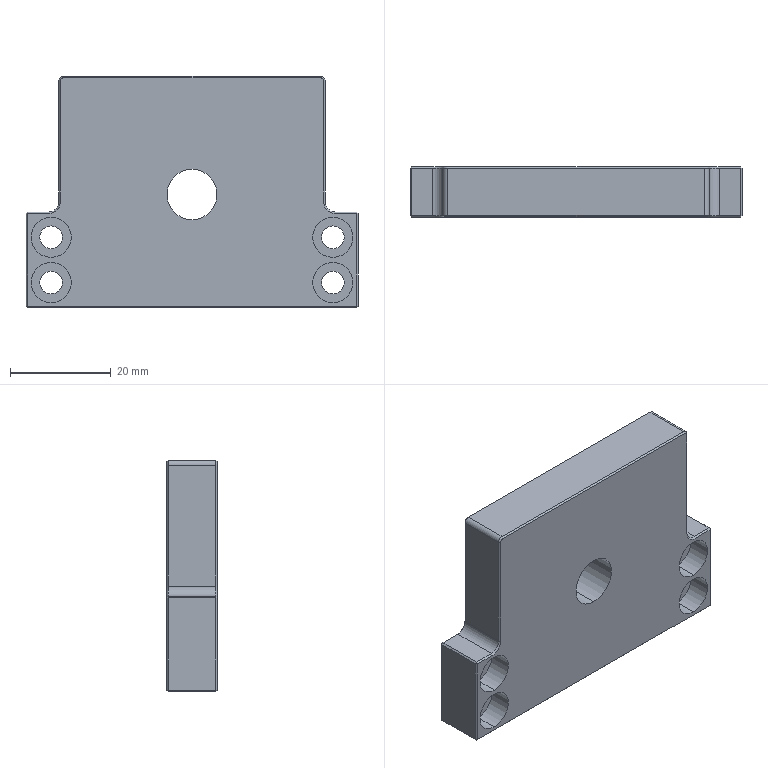Part | SolidWorks | features BaseBody 1 | 1 solid | 72 faces | box 66 x 10 x 46 mm | volume 24787 mm3 | plane 42 | cylinder 22 | cone 8 | commonest cylinder face diameters 4.5 x8 8 x8 2 x2 4 x2 10 x2